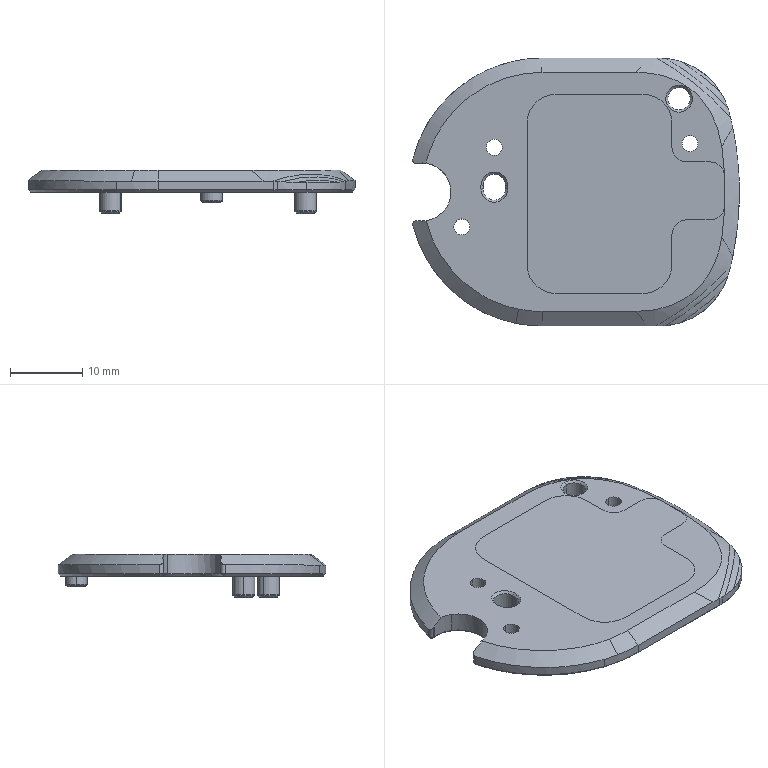NC program | NX | posted with a generic post | part box 45.101 x 36.973 x 6 mm
Lines 1 to 1808 of 5084, first 1683 of 1794 lines:
N10 G17 G21 G94 G90
(FLOOR_WALL_COPY_COPY , TOOL : D80)
N12 T19 M6
N14 G54
N16 G17 G0 G90 X-67.55 Y0. S6500 M3
N18 G43 Z30. H19
N20 Z6.
N22 G94 G1 Z3. F1500.
N24 X-62.55
N26 X62.55
N28 X67.55
N30 Z6.
N32 G0 Z30.
N34 X-67.55
N36 Z5.
N38 G1 Z2.
N40 X-62.55
N42 X62.55
N44 X67.55
N46 Z5.
N48 G0 Z30.
N50 X-67.55
N52 Z4.
N54 G1 Z1.
N56 X-62.55
N58 X62.55
N60 X67.55
N62 Z4.
N64 G0 Z30.
N66 X-67.55
N68 Z3.
N70 G1 Z0.
N72 X-62.55
N74 X62.55
N76 X67.55
N78 Z3.
N80 G0 Z30.
N82 M5
(CAVITY_MILL , TOOL : D6)
N84 T12 M6
N86 G54
N88 G17 G0 G90 X0.167 Y22.684 S9500 M3
N90 G43 Z30. H12
N92 Z0.65
N94 G94 G1 Z-0.35 F1000.
N96 Y18.831
N98 G3 X0.379 Y18.784 R0.5
N100 G1 X15.035 F3000.
N102 G2 X22.848 Y11.359 R21.5
N104 G1 Y1.003
N106 G2 X21.428 Y0.967 R3.5
N108 G3 X21.428 Y-1.001 R-1.
N110 G2 X22.848 Y-1.038 R3.5
N112 G1 Y-11.39
N114 G2 X15.091 Y-18.784 R21.5
N116 G1 X-19.432
N118 G2 X-22.848 Y-14.792 R13.
N120 G1 Y14.761
N122 G2 X-19.395 Y18.784 R13.
N124 G1 X0.379
N126 Y15.184
N128 X14.057
N130 G2 X19.248 Y10.277 R17.9
N132 G1 Y4.124
N134 G3 X19.248 Y-4.158 R4.6
N136 G1 Y-10.308
N138 G2 X14.107 Y-15.184 R17.9
N140 G1 X13.847
N142 G3 X8.65 Y-15.184 R-5.318
N144 G1 X9.002 Y-14.556
N146 G2 X7.237 Y-8.297 R4.598
N148 X9.002 Y-14.556 R-4.598
N150 G1 X8.65 Y-15.184
N152 X-18.086
N154 G2 X-19.248 Y-13.784 R9.4
N156 G1 Y-11.086
N158 G3 X-11.16 Y-9.945 R5.318
N160 X-10.588 Y-8.675 R5.318
N162 G1 X-10.437 Y-8.039
N164 G3 X-10.406 Y-7.825 R5.318
N166 G1 X-10.362 Y-7.253
N168 G3 X-19.248 Y-3.199 R5.318
N170 G1 X-18.765 Y-3.733
N172 G2 X-11.082 Y-7.238 R4.598
N174 G1 X-11.124 Y-7.769
N176 X-11.147 Y-7.917
N178 X-11.288 Y-8.507
N180 G2 X-18.765 Y-3.733 R-4.598
N182 G1 X-19.248 Y-3.199
N184 Y13.753
N186 G2 X-18.057 Y15.184 R9.4
N188 G1 X0.379
N190 Y11.584
N192 X12.966
N194 G2 X15.648 Y9.068 R14.3
N196 G1 Y5.97
N198 G3 X13.259 Y-1.855 R8.2
N200 X2.391 Y-11.584 R8.918
N202 G1 X-7.946
N204 G3 X-7.111 Y-9.612 R8.918
N206 G1 X-6.932 Y-8.867
N208 X-6.899 Y-8.704
N210 G3 X-6.837 Y-8.306 R8.918
N212 G1 X-6.821 Y-8.161
N214 X-6.771 Y-7.526
N216 X-6.764 Y-7.381
N218 G3 X-6.762 Y-7.013 R8.918
N220 X-15.648 Y1.776 R8.918
N222 G1 Y11.584
N224 X0.379
N226 Y7.984
N228 X11.709
N230 G2 X12.048 Y7.67 R10.7
N232 G1 Y7.368
N234 G3 X9.602 Y1.866 R11.8
N236 X-1.005 Y-7.984 R12.518
N238 G1 X-3.196
N240 X-3.178 Y-7.758
N242 X-3.166 Y-7.518
N244 G3 X-3.162 Y-6.959 R12.518
N246 X-12.048 Y4.838 R12.518
N248 G1 Y7.984
N250 X0.379
N252 Y4.384
N254 X5.17
N256 G3 X-1.126 Y-0.215 R16.118
N258 X-4.412 Y4.384 R16.118
N260 G1 X0.379
N262 G3 X1.145 Y4.741 R1.
N264 G1 Z0.65
N266 G0 Z30.
N268 X0.166 Y22.684
N270 Z0.3
N272 G1 Z-0.7 F1000.
N274 Y18.831
N276 G3 X0.378 Y18.784 R0.5
N278 G1 X15.035 F3000.
N280 G2 X22.848 Y11.359 R21.5
N282 G1 Y1.003
N284 G2 X21.428 Y0.967 R3.5
N286 G3 X21.428 Y-1.001 R-1.
N288 G2 X22.848 Y-1.038 R3.5
N290 G1 Y-11.39
N292 G2 X15.09 Y-18.784 R21.5
N294 G1 X-19.432
N296 G2 X-22.848 Y-14.792 R13.
N298 G1 Y14.761
N300 G2 X-19.395 Y18.784 R13.
N302 G1 X0.378
N304 Y15.184
N306 X14.057
N308 G2 X19.248 Y10.277 R17.9
N310 G1 Y4.124
N312 G3 X19.248 Y-4.158 R4.6
N314 G1 Y-10.308
N316 G2 X14.107 Y-15.184 R17.9
N318 G1 X13.85
N320 G3 X8.647 Y-15.184 R-5.32
N322 G1 X8.999 Y-14.556
N324 G2 X7.236 Y-8.294 R4.6
N326 X8.999 Y-14.556 R-4.6
N328 G1 X8.647 Y-15.184
N330 X-18.086
N332 G2 X-19.248 Y-13.783 R9.4
N334 G1 Y-11.088
N336 G3 X-19.248 Y-3.196 R-5.32
N338 G1 X-18.765 Y-3.73
N340 G2 X-12.268 Y-4.057 R4.6
N342 X-18.765 Y-3.73 R-4.6
N344 G1 X-19.248 Y-3.196
N346 Y13.753
N348 G2 X-18.056 Y15.184 R9.4
N350 G1 X0.378
N352 Y11.584
N354 X12.966
N356 G2 X15.648 Y9.068 R14.3
N358 G1 Y5.97
N360 G3 X13.259 Y-1.853 R8.2
N362 X2.389 Y-11.584 R8.92
N364 G1 X-7.944
N366 G3 X-15.648 Y1.778 R8.92
N368 G1 Y11.584
N370 X0.378
N372 Y7.984
N374 X11.709
N376 G2 X12.048 Y7.67 R10.7
N378 G1 Y7.369
N380 G3 X9.602 Y1.867 R11.8
N382 X-1.007 Y-7.984 R12.52
N384 G1 X-3.188
N386 G3 X-12.048 Y4.84 R12.52
N388 G1 Y7.984
N390 X0.378
N392 Y4.384
N394 X5.165
N396 G3 X-1.125 Y-0.212 R16.12
N398 X-4.41 Y4.384 R16.12
N400 G1 X0.378
N402 G3 X1.144 Y4.741 R1.
N404 G1 Z0.3
N406 G0 X0.166 Y22.684 Z-0.05
N408 G1 Z-1.05 F1000.
N410 Y18.831
N412 G3 X0.378 Y18.784 R0.5
N414 G1 X15.035 F3000.
N416 G2 X22.848 Y11.359 R21.5
N418 G1 Y1.003
N420 G2 X21.428 Y0.967 R3.5
N422 G3 X21.428 Y-1.001 R-1.
N424 G2 X22.848 Y-1.038 R3.5
N426 G1 Y-11.39
N428 G2 X15.09 Y-18.784 R21.5
N430 G1 X-19.432
N432 G2 X-22.848 Y-14.791 R13.
N434 G1 Y14.761
N436 G2 X-19.395 Y18.784 R13.
N438 G1 X0.378
N440 Y15.184
N442 X14.057
N444 G2 X19.248 Y10.277 R17.9
N446 G1 Y4.124
N448 G3 X19.248 Y-4.159 R4.6
N450 G1 Y-10.308
N452 G2 X14.106 Y-15.184 R17.9
N454 G1 X13.85
N456 G3 X8.647 Y-15.184 R-5.32
N458 G1 X8.999 Y-14.556
N460 G2 X7.236 Y-8.294 R4.6
N462 X8.999 Y-14.556 R-4.6
N464 G1 X8.647 Y-15.184
N466 X-18.086
N468 G2 X-19.248 Y-13.783 R9.4
N470 G1 Y-11.088
N472 G3 X-19.248 Y-3.197 R-5.32
N474 G1 X-18.765 Y-3.731
N476 G2 X-12.268 Y-4.057 R4.6
N478 X-18.765 Y-3.731 R-4.6
N480 G1 X-19.248 Y-3.197
N482 Y13.753
N484 G2 X-18.056 Y15.184 R9.4
N486 G1 X0.378
N488 Y11.584
N490 X12.966
N492 G2 X15.648 Y9.067 R14.3
N494 G1 Y5.97
N496 G3 X13.259 Y-1.853 R8.2
N498 X2.389 Y-11.584 R8.92
N500 G1 X-7.944
N502 G3 X-15.648 Y1.778 R8.92
N504 G1 Y11.584
N506 X0.378
N508 Y7.984
N510 X11.709
N512 G2 X12.048 Y7.67 R10.7
N514 G1 Y7.369
N516 G3 X9.602 Y1.867 R11.8
N518 X-1.007 Y-7.984 R12.52
N520 G1 X-3.188
N522 G3 X-12.048 Y4.84 R12.52
N524 G1 Y7.984
N526 X0.378
N528 Y4.384
N530 X5.165
N532 G3 X-1.125 Y-0.212 R16.12
N534 X-4.41 Y4.384 R16.12
N536 G1 X0.378
N538 G3 X1.144 Y4.742 R1.
N540 G1 Z-0.05
N542 G0 X0.166 Y22.684 Z-0.4
N544 G1 Z-1.4 F1000.
N546 Y18.831
N548 G3 X0.378 Y18.784 R0.5
N550 G1 X15.034 F3000.
N552 G2 X22.848 Y11.358 R21.5
N554 G1 Y1.003
N556 G2 X21.428 Y0.967 R3.5
N558 G3 X21.428 Y-1.001 R-1.
N560 G2 X22.848 Y-1.038 R3.5
N562 G1 Y-11.389
N564 G2 X15.09 Y-18.784 R21.5
N566 G1 X-19.432
N568 G2 X-22.848 Y-14.791 R13.
N570 G1 Y14.76
N572 G2 X-19.394 Y18.784 R13.
N574 G1 X0.378
N576 Y15.184
N578 X14.057
N580 G2 X19.248 Y10.277 R17.9
N582 G1 Y4.124
N584 G3 X19.248 Y-4.159 R4.6
N586 G1 Y-10.308
N588 G2 X14.106 Y-15.184 R17.9
N590 G1 X13.85
N592 G3 X8.647 Y-15.184 R-5.32
N594 G1 X8.999 Y-14.556
N596 G2 X7.236 Y-8.295 R4.6
N598 X8.999 Y-14.556 R-4.6
N600 G1 X8.647 Y-15.184
N602 X-18.086
N604 G2 X-19.248 Y-13.783 R9.4
N606 G1 Y-11.088
N608 G3 X-19.248 Y-3.197 R-5.32
N610 G1 X-18.765 Y-3.731
N612 G2 X-12.268 Y-4.056 R4.6
N614 X-18.765 Y-3.731 R-4.6
N616 G1 X-19.248 Y-3.197
N618 Y13.753
N620 G2 X-18.056 Y15.184 R9.4
N622 G1 X0.378
N624 Y11.584
N626 X12.966
N628 G2 X15.648 Y9.067 R14.3
N630 G1 Y5.97
N632 G3 X13.259 Y-1.853 R8.2
N634 X2.389 Y-11.584 R8.92
N636 G1 X-7.944
N638 G3 X-15.648 Y1.778 R8.92
N640 G1 Y11.584
N642 X0.378
N644 Y7.984
N646 X11.709
N648 G2 X12.048 Y7.67 R10.7
N650 G1 Y7.369
N652 G3 X9.602 Y1.867 R11.8
N654 X-1.007 Y-7.984 R12.52
N656 G1 X-3.188
N658 G3 X-12.048 Y4.84 R12.52
N660 G1 Y7.984
N662 X0.378
N664 Y4.384
N666 X5.166
N668 G3 X-1.125 Y-0.212 R16.12
N670 X-4.41 Y4.384 R16.12
N672 G1 X0.378
N674 G3 X1.144 Y4.742 R1.
N676 G1 Z-0.4
N678 G0 X-1.96 Y-22.685 Z-0.775
N680 G1 Z-1.775 F1000.
N682 Y-18.831
N684 G3 X-2.171 Y-18.785 R0.5
N686 G1 X-19.431 F3000.
N688 G2 X-22.848 Y-14.791 R13.
N690 G1 Y14.76
N692 G2 X-19.394 Y18.785 R13.
N694 G1 X-7.207
N696 G2 X1.794 Y18.785 R5.3
N698 G1 X15.034
N700 G2 X22.848 Y11.358 R21.5
N702 G1 Y1.003
N704 G2 X21.428 Y0.967 R3.5
N706 G3 X21.428 Y-1.001 R-1.
N708 G2 X22.848 Y-1.038 R3.5
N710 G1 Y-11.389
N712 G2 X15.09 Y-18.785 R21.5
N714 G1 X-2.171
N716 Y-15.185
N718 X-18.086
N720 G2 X-19.248 Y-13.783 R9.4
N722 G1 Y-11.088
N724 G3 X-19.248 Y-3.197 R-5.32
N726 G1 X-18.765 Y-3.731
N728 G2 X-12.268 Y-4.056 R4.6
N730 X-18.765 Y-3.731 R-4.6
N732 G1 X-19.248 Y-3.197
N734 Y13.753
N736 G2 X-18.056 Y15.185 R9.4
N738 G1 X-7.946
N740 G3 X2.533 Y15.185 R5.3
N742 G1 X1.821 Y15.293
N744 G2 X-3.398 Y11.458 R4.58
N746 X1.821 Y15.293 R-4.58
N748 G1 X2.533 Y15.185
N750 X14.056
N752 G2 X19.248 Y10.276 R17.9
N754 G1 Y4.124
N756 G3 X19.248 Y-4.159 R4.6
N758 G1 Y-10.307
N760 G2 X14.106 Y-15.185 R17.9
N762 G1 X13.85
N764 G3 X8.647 Y-15.185 R-5.32
N766 G1 X8.999 Y-14.557
N768 G2 X7.236 Y-8.295 R4.6
N770 X8.999 Y-14.557 R-4.6
N772 G1 X8.647 Y-15.185
N774 X-2.171
N776 Y-11.585
N778 X-7.944
N780 G3 X-15.648 Y1.778 R8.92
N782 G1 Y11.585
N784 X-10.443
N786 G3 X5.029 Y11.585 R8.9
N788 G1 X12.965
N790 G2 X15.648 Y9.067 R14.3
N792 G1 Y5.971
N794 G3 X13.259 Y-1.853 R8.2
N796 X2.389 Y-11.585 R8.92
N798 G1 X-2.171
N800 Y-7.985
N802 X-3.188
N804 G3 X-12.048 Y4.84 R12.52
N806 G1 Y7.68
N808 G3 X6.898 Y7.985 R12.5
N810 G1 X11.709
N812 G2 X12.048 Y7.669 R10.7
N814 G1 Y7.369
N816 G3 X9.602 Y1.867 R11.8
N818 X-1.007 Y-7.985 R12.52
N820 G1 X-2.171
N822 X-1.125 Y-0.212
N824 X-1.206 Y-0.045
N826 G3 X-0.962 Y-0.02 R16.1
N828 X-1.125 Y-0.212 R16.12
N830 X-1.342 Y-1.029 R1.
N832 G1 Z-0.775
N834 G0 X-1.96 Y-22.685 Z-1.15
N836 G1 Z-2.15 F1000.
N838 Y-18.832
N840 G3 X-2.171 Y-18.785 R0.5
N842 G1 X-19.431 F3000.
N844 G2 X-22.849 Y-14.79 R13.
N846 G1 Y14.76
N848 G2 X-19.394 Y18.785 R13.
N850 G1 X-7.23
N852 G2 X1.817 Y18.785 R5.32
N854 G1 X15.034
N856 G2 X22.849 Y11.358 R21.5
N858 G1 Y1.003
N860 G2 X21.428 Y0.967 R3.5
N862 G3 X21.428 Y-1.001 R-1.
N864 G2 X22.849 Y-1.038 R3.5
N866 G1 Y-11.389
N868 G2 X15.089 Y-18.785 R21.5
N870 G1 X-2.171
N872 Y-15.185
N874 X-18.085
N876 G2 X-19.249 Y-13.782 R9.4
N878 G1 Y-11.088
N880 G3 X-19.249 Y-3.197 R-5.32
N882 G1 X-18.766 Y-3.731
N884 G2 X-12.268 Y-4.056 R4.6
N886 X-18.766 Y-3.731 R-4.6
N888 G1 X-19.249 Y-3.197
N890 Y13.752
N892 G2 X-18.056 Y15.185 R9.4
N894 G1 X-7.966
N896 G3 X2.553 Y15.185 R5.32
N898 G1 X1.841 Y15.293
N900 G2 X-3.399 Y11.437 R4.6
N902 X1.841 Y15.293 R-4.6
N904 G1 X2.553 Y15.185
N906 X14.056
N908 G2 X19.249 Y10.276 R17.9
N910 G1 Y4.124
N912 G3 X19.249 Y-4.159 R4.6
N914 G1 Y-10.307
N916 G2 X14.106 Y-15.185 R17.9
N918 G1 X13.849
N920 G3 X8.648 Y-15.185 R-5.32
N922 G1 X9. Y-14.557
N924 G2 X7.236 Y-8.295 R4.6
N926 X9. Y-14.557 R-4.6
N928 G1 X8.648 Y-15.185
N930 X-2.171
N932 Y-11.585
N934 X-7.944
N936 G3 X-15.649 Y1.778 R8.92
N938 G1 Y11.585
N940 X-10.466
N942 G3 X5.053 Y11.585 R8.92
N944 G1 X12.965
N946 G2 X15.649 Y9.067 R14.3
N948 G1 Y5.971
N950 G3 X13.259 Y-1.853 R8.2
N952 X2.389 Y-11.585 R8.92
N954 G1 X-2.171
N956 Y-7.985
N958 X-3.188
N960 G3 X-12.049 Y4.84 R12.52
N962 G1 Y7.65
N964 G3 X6.924 Y7.985 R12.52
N966 G1 X11.708
N968 G2 X12.049 Y7.669 R10.7
N970 G1 Y7.369
N972 G3 X9.602 Y1.867 R11.8
N974 X-1.007 Y-7.985 R12.52
N976 G1 X-2.171
N978 X-1.125 Y-0.212
N980 X-1.196 Y-0.064
N982 G3 X-0.982 Y-0.042 R16.12
N984 X-1.125 Y-0.212 R16.12
N986 X-1.342 Y-1.029 R1.
N988 G1 Z-1.15
N990 G0 X-1.96 Y-22.685 Z-1.525
N992 G1 Z-2.525 F1000.
N994 Y-18.832
N996 G3 X-2.171 Y-18.785 R0.5
N998 G1 X-19.431 F3000.
N1000 G2 X-22.849 Y-14.79 R13.
N1002 G1 Y14.759
N1004 G2 X-19.394 Y18.785 R13.
N1006 G1 X-7.23
N1008 G2 X1.817 Y18.785 R5.32
N1010 G1 X15.034
N1012 G2 X22.849 Y11.358 R21.5
N1014 G1 Y1.003
N1016 G2 X21.428 Y0.967 R3.5
N1018 G3 X21.428 Y-1.001 R-1.
N1020 G2 X22.849 Y-1.038 R3.5
N1022 G1 Y-11.388
N1024 G2 X15.089 Y-18.785 R21.5
N1026 G1 X-2.171
N1028 Y-15.185
N1030 X-18.085
N1032 G2 X-19.249 Y-13.782 R9.4
N1034 G1 Y-11.087
N1036 G3 X-19.249 Y-3.197 R-5.32
N1038 G1 X-18.766 Y-3.731
N1040 G2 X-12.268 Y-4.056 R4.6
N1042 X-18.766 Y-3.731 R-4.6
N1044 G1 X-19.249 Y-3.197
N1046 Y13.752
N1048 G2 X-18.056 Y15.185 R9.4
N1050 G1 X-7.966
N1052 G3 X2.553 Y15.185 R5.32
N1054 G1 X1.841 Y15.293
N1056 G2 X-3.398 Y11.437 R4.6
N1058 X1.841 Y15.293 R-4.6
N1060 G1 X2.553 Y15.185
N1062 X14.056
N1064 G2 X19.249 Y10.276 R17.9
N1066 G1 Y4.124
N1068 G3 X19.249 Y-4.159 R4.6
N1070 G1 Y-10.307
N1072 G2 X14.106 Y-15.185 R17.9
N1074 G1 X13.849
N1076 G3 X8.648 Y-15.185 R-5.32
N1078 G1 X9. Y-14.557
N1080 G2 X7.236 Y-8.295 R4.6
N1082 X9. Y-14.557 R-4.6
N1084 G1 X8.648 Y-15.185
N1086 X-2.171
N1088 Y-11.585
N1090 X-7.944
N1092 G3 X-15.649 Y1.778 R8.92
N1094 G1 Y11.585
N1096 X-10.466
N1098 G3 X5.053 Y11.585 R8.92
N1100 G1 X12.965
N1102 G2 X15.649 Y9.067 R14.3
N1104 G1 Y5.971
N1106 G3 X13.259 Y-1.853 R8.2
N1108 X2.389 Y-11.585 R8.92
N1110 G1 X-2.171
N1112 Y-7.985
N1114 X-3.188
N1116 G3 X-12.049 Y4.84 R12.52
N1118 G1 Y7.65
N1120 G3 X6.924 Y7.985 R12.52
N1122 G1 X11.708
N1124 G2 X12.049 Y7.669 R10.7
N1126 G1 Y7.37
N1128 G3 X9.602 Y1.867 R11.8
N1130 X-1.007 Y-7.985 R12.52
N1132 G1 X-2.171
N1134 X-1.125 Y-0.212
N1136 X-1.196 Y-0.064
N1138 G3 X-0.982 Y-0.042 R16.12
N1140 X-1.125 Y-0.212 R16.12
N1142 X-1.342 Y-1.029 R1.
N1144 G1 Z-1.525
N1146 G0 X-1.96 Y-22.685 Z-1.9
N1148 G1 Z-2.9 F1000.
N1150 Y-18.832
N1152 G3 X-2.171 Y-18.785 R0.5
N1154 G1 X-19.431 F3000.
N1156 G2 X-22.849 Y-14.79 R13.
N1158 G1 Y14.759
N1160 G2 X-19.394 Y18.785 R13.
N1162 G1 X-7.23
N1164 G2 X1.817 Y18.785 R5.32
N1166 G1 X15.033
N1168 G2 X22.849 Y11.357 R21.5
N1170 G1 Y1.003
N1172 G2 X21.428 Y0.967 R3.5
N1174 G3 X21.428 Y-1.001 R-1.
N1176 G2 X22.849 Y-1.038 R3.5
N1178 G1 Y-11.388
N1180 G2 X15.089 Y-18.785 R21.5
N1182 G1 X-2.171
N1184 Y-15.185
N1186 X-18.085
N1188 G2 X-19.249 Y-13.782 R9.4
N1190 G1 Y-11.087
N1192 G3 X-19.249 Y-3.197 R-5.32
N1194 G1 X-18.766 Y-3.731
N1196 G2 X-12.268 Y-4.056 R4.6
N1198 X-18.766 Y-3.731 R-4.6
N1200 G1 X-19.249 Y-3.197
N1202 Y13.752
N1204 G2 X-18.056 Y15.185 R9.4
N1206 G1 X-7.966
N1208 G3 X2.553 Y15.185 R5.32
N1210 G1 X1.841 Y15.293
N1212 G2 X-3.398 Y11.437 R4.6
N1214 X1.841 Y15.293 R-4.6
N1216 G1 X2.553 Y15.185
N1218 X14.056
N1220 G2 X19.249 Y10.276 R17.9
N1222 G1 Y4.124
N1224 G3 X19.249 Y-4.159 R4.6
N1226 G1 Y-10.307
N1228 G2 X14.105 Y-15.185 R17.9
N1230 G1 X13.849
N1232 G3 X8.648 Y-15.185 R-5.32
N1234 G1 X9. Y-14.557
N1236 G2 X7.235 Y-8.295 R4.6
N1238 X9. Y-14.557 R-4.6
N1240 G1 X8.648 Y-15.185
N1242 X-2.171
N1244 Y-11.585
N1246 X-7.944
N1248 G3 X-15.649 Y1.778 R8.92
N1250 G1 Y11.585
N1252 X-10.466
N1254 G3 X5.053 Y11.585 R8.92
N1256 G1 X12.965
N1258 G2 X15.649 Y9.066 R14.3
N1260 G1 Y5.971
N1262 G3 X13.259 Y-1.853 R8.2
N1264 X2.389 Y-11.585 R8.92
N1266 G1 X-2.171
N1268 Y-7.985
N1270 X-3.188
N1272 G3 X-12.049 Y4.84 R12.52
N1274 G1 Y7.65
N1276 G3 X6.924 Y7.985 R12.52
N1278 G1 X11.708
N1280 G2 X12.049 Y7.669 R10.7
N1282 G1 Y7.37
N1284 G3 X9.602 Y1.867 R11.8
N1286 X-1.007 Y-7.985 R12.52
N1288 G1 X-2.171
N1290 X-1.125 Y-0.212
N1292 X-1.196 Y-0.064
N1294 G3 X-0.982 Y-0.042 R16.12
N1296 X-1.125 Y-0.212 R16.12
N1298 X-1.342 Y-1.029 R1.
N1300 G1 Z-1.9
N1302 G0 X-3.718 Y-2.069 Z-1.4
N1304 G1 X-3.562 Y-2.478 Z-1.423 F1000.
N1306 X-3.384 Y-3.313 Z-1.468
N1308 Y3.351 Z-1.817
N1310 X-3.443 Z-1.82
N1312 X-3.641 Y2.52 Z-1.865
N1314 X-4.281 Y0.893 Z-1.956
N1316 X-4.703 Y0.151 Z-2.001
N1318 X-4.281 Y-0.591 Z-2.046
N1320 X-3.562 Y-2.478 Z-2.152
N1322 X-3.384 Y-3.313 Z-2.197
N1324 Y3.351 Z-2.546
N1326 X-3.443 Z-2.549
N1328 X-3.641 Y2.52 Z-2.594
N1330 X-4.281 Y0.893 Z-2.685
N1332 X-4.703 Y0.151 Z-2.73
N1334 X-4.281 Y-0.591 Z-2.775
N1336 X-3.562 Y-2.478 Z-2.881
N1338 X-3.384 Y-3.313 Z-2.925
N1340 Y0.019 Z-3.1
N1342 Y3.351 F3000.
N1344 X-3.443
N1346 G2 X-4.703 Y0.151 R12.134
N1348 X-3.384 Y-3.313 R12.134
N1350 G1 Y0.019
N1352 X0.216
N1354 Y6.951
N1356 X-6.716
N1358 Y6.151
N1360 G2 X-9.181 Y0.151 R8.534
N1362 X-6.716 Y-5.849 R8.534
N1364 G1 Y-7.937
N1366 G2 X-4.182 Y-7.481 R7.006
N1368 G1 X0.216
N1370 Y0.019
N1372 X3.816
N1374 Y9.475
N1376 G3 X2.733 Y10.551 R1.066
N1378 G1 X-9.24
N1380 G3 X-10.316 Y9.485 R1.066
N1382 G1 Y6.151
N1384 G2 X-15.25 Y1.217 R4.934
N1386 G1 X-17.58 Y1.218
N1388 Y-0.914
N1390 X-15.249 Y-0.915
N1392 G2 X-10.316 Y-5.849 R4.934
N1394 G1 Y-10.015
N1396 X-10.277 Y-10.483
N1398 G2 X-12.204 Y-13.802 R3.352
N1400 G1 X-7.551 Y-13.731
N1402 G2 X-4.196 Y-11.081 R3.406
N1404 G1 X2.75
N1406 G3 X3.816 Y-10.034 R1.066
N1408 G1 Y0.019
N1410 G3 X3.459 Y0.785 R1.
N1412 G1 Z-2.1
N1414 G0 X-3.55 Y1.045 Z-1.6
N1416 G1 Y2.357 Z-1.669 F1000.
N1418 X-3.815 Y1.539 Z-1.714
N1420 X-4.093 Y0.902 Z-1.75
N1422 X-4.512 Y0.151 Z-1.795
N1424 X-4.093 Y-0.599 Z-1.84
N1426 X-3.815 Y-1.236 Z-1.877
N1428 X-3.55 Y-2.054 Z-1.922
N1430 Y2.357 Z-2.153
N1432 X-3.815 Y1.539 Z-2.198
N1434 X-4.093 Y0.902 Z-2.234
N1436 X-4.512 Y0.151 Z-2.279
N1438 X-4.093 Y-0.599 Z-2.325
N1440 X-3.815 Y-1.236 Z-2.361
N1442 X-3.55 Y-2.054 Z-2.406
N1444 Y2.357 Z-2.637
N1446 X-3.815 Y1.539 Z-2.682
N1448 X-4.093 Y0.902 Z-2.719
N1450 X-4.512 Y0.151 Z-2.764
N1452 X-4.093 Y-0.599 Z-2.809
N1454 X-3.815 Y-1.236 Z-2.845
N1456 X-3.55 Y-2.054 Z-2.89
N1458 Y2.357 Z-3.121
N1460 X-3.815 Y1.539 Z-3.166
N1462 X-4.093 Y0.902 Z-3.203
N1464 X-4.512 Y0.151 Z-3.248
N1466 X-4.093 Y-0.599 Z-3.293
N1468 X-3.815 Y-1.236 Z-3.329
N1470 X-3.55 Y-2.054 Z-3.374
N1472 Y0.151 Z-3.49
N1474 Y2.357 F3000.
N1476 G2 X-4.512 Y0.151 R12.3
N1478 X-3.55 Y-2.054 R12.3
N1480 G1 Y0.151
N1482 X0.05
N1484 Y6.785
N1486 X-6.55
N1488 Y6.141
N1490 G2 X-8.95 Y0.151 R8.7
N1492 X-6.55 Y-5.836 R8.7
N1494 G1 Y-7.684
N1496 G2 X-4.443 Y-7.316 R6.995
N1498 G1 X0.05 Y-7.315
N1500 Y0.151
N1502 X3.65
N1504 Y9.485
N1506 G3 X2.75 Y10.385 R0.9
N1508 G1 X-9.25
N1510 G3 X-10.15 Y9.485 R0.9
N1512 G1 Y6.143
N1514 G2 X-15.25 Y1.051 R5.1
N1516 G1 X-17.414 Y1.052
N1518 Y-0.748
N1520 X-15.233 Y-0.749
N1522 G2 X-10.15 Y-5.84 R5.1
N1524 G1 Y-10.015
N1526 X-10.134 Y-10.184
N1528 G2 X-11.381 Y-13.565 R3.587
N1530 G1 X-7.742 Y-13.509
N1532 G2 X-6.644 Y-11.847 R3.168
N1534 X-4.373 Y-10.915 R3.395
N1536 G1 X2.75
N1538 G3 X3.65 Y-10.015 R0.9
N1540 G1 Y0.151
N1542 G3 X3.293 Y0.917 R1.
N1544 G1 Z-2.49
N1546 G0 X-3.55 Y1.045 Z-1.99
N1548 G1 Y2.357 Z-2.059 F1000.
N1550 X-3.815 Y1.539 Z-2.104
N1552 X-4.093 Y0.902 Z-2.14
N1554 X-4.512 Y0.151 Z-2.185
N1556 X-4.093 Y-0.599 Z-2.23
N1558 X-3.815 Y-1.236 Z-2.267
N1560 X-3.55 Y-2.054 Z-2.312
N1562 Y2.357 Z-2.543
N1564 X-3.815 Y1.539 Z-2.588
N1566 X-4.093 Y0.902 Z-2.624
N1568 X-4.512 Y0.151 Z-2.669
N1570 X-4.093 Y-0.599 Z-2.715
N1572 X-3.815 Y-1.236 Z-2.751
N1574 X-3.55 Y-2.054 Z-2.796
N1576 Y2.357 Z-3.027
N1578 X-3.815 Y1.539 Z-3.072
N1580 X-4.093 Y0.902 Z-3.109
N1582 X-4.512 Y0.151 Z-3.154
N1584 X-4.093 Y-0.599 Z-3.199
N1586 X-3.815 Y-1.236 Z-3.235
N1588 X-3.55 Y-2.054 Z-3.28
N1590 Y2.357 Z-3.511
N1592 X-3.815 Y1.539 Z-3.556
N1594 X-4.093 Y0.902 Z-3.593
N1596 X-4.512 Y0.151 Z-3.638
N1598 X-4.093 Y-0.599 Z-3.683
N1600 X-3.815 Y-1.236 Z-3.719
N1602 X-3.55 Y-2.054 Z-3.764
N1604 Y0.151 Z-3.88
N1606 Y2.357 F3000.
N1608 G2 X-4.512 Y0.151 R12.3
N1610 X-3.55 Y-2.054 R12.3
N1612 G1 Y0.151
N1614 X0.05
N1616 Y6.785
N1618 X-6.55
N1620 Y6.141
N1622 G2 X-8.95 Y0.151 R8.7
N1624 X-6.55 Y-5.836 R8.7
N1626 G1 Y-7.611
N1628 G2 X-5.145 Y-7.339 R8.161
N1630 G1 X0.05 Y-7.315
N1632 Y0.151
N1634 X3.65
N1636 Y9.485
N1638 G3 X2.75 Y10.385 R0.9
N1640 G1 X-9.25
N1642 G3 X-10.15 Y9.485 R0.9
N1644 G1 Y6.143
N1646 G2 X-15.25 Y1.051 R5.1
N1648 G1 X-17.414 Y1.052
N1650 Y-0.748
N1652 X-15.233 Y-0.749
N1654 G2 X-10.15 Y-5.84 R5.1
N1656 G1 Y-10.015
N1658 G3 X-10.122 Y-10.236 R0.9
N1660 G2 X-10.112 Y-11.963 R3.522
N1662 G1 X-10.333 Y-12.923
N1664 X-8.076 Y-12.888
N1666 G2 X-4.847 Y-10.929 R4.561
N1668 G1 X-4.548 Y-10.915
N1670 X2.75
N1672 G3 X3.65 Y-10.015 R0.9
N1674 G1 Y0.151
N1676 G3 X3.293 Y0.917 R1.
N1678 G1 Z-2.88
N1680 G0 X-3.939 Y1.255 Z-2.38
N1682 G1 X-4.093 Y0.902 Z-2.4 F1000.
N1684 X-4.512 Y0.151 Z-2.445
N1686 X-4.093 Y-0.599 Z-2.49
N1688 X-3.815 Y-1.236 Z-2.527
N1690 X-3.55 Y-2.054 Z-2.572
N1692 Y2.357 Z-2.803
N1694 X-3.815 Y1.539 Z-2.848
N1696 X-4.093 Y0.902 Z-2.884
N1698 X-4.512 Y0.151 Z-2.929
N1700 X-4.093 Y-0.599 Z-2.975
N1702 X-3.815 Y-1.236 Z-3.011
N1704 X-3.55 Y-2.054 Z-3.056
N1706 Y2.357 Z-3.287
N1708 X-3.815 Y1.539 Z-3.332
N1710 X-4.093 Y0.902 Z-3.369
N1712 X-4.512 Y0.151 Z-3.414
N1714 X-4.093 Y-0.599 Z-3.459
N1716 X-3.815 Y-1.236 Z-3.495
N1718 X-3.55 Y-2.054 Z-3.54
N1720 Y2.357 Z-3.771
N1722 X-3.815 Y1.539 Z-3.816
N1724 X-4.093 Y0.902 Z-3.853
N1726 X-4.512 Y0.151 Z-3.898
N1728 X-4.093 Y-0.599 Z-3.943
N1730 X-3.815 Y-1.236 Z-3.979
N1732 X-3.55 Y-2.054 Z-4.024
N1734 Y0.151 Z-4.14
N1736 Y2.357 F3000.
N1738 G2 X-4.512 Y0.151 R12.3
N1740 X-3.55 Y-2.054 R12.3
N1742 G1 Y0.151
N1744 X0.05
N1746 Y6.785
N1748 X-6.55
N1750 Y6.141
N1752 G2 X-8.95 Y0.151 R8.7
N1754 X-6.55 Y-5.836 R8.7
N1756 G1 Y-7.414
N1758 X-6.138
N1760 X-5.009 Y-7.315
N1762 X0.05
N1764 Y0.151
N1766 X3.65
N1768 Y9.485
N1770 G3 X2.75 Y10.385 R0.9
N1772 G1 X-9.25
N1774 G3 X-10.15 Y9.485 R0.9
N1776 G1 Y6.143
N1778 G2 X-15.25 Y1.051 R5.1
N1780 G1 X-17.414 Y1.052
N1782 Y-0.748
N1784 X-15.233 Y-0.749
N1786 G2 X-10.15 Y-5.84 R5.1
N1788 G1 Y-10.015
N1790 G3 X-10.106 Y-10.301 R0.903
N1792 G1 X-9.993 Y-10.682
N1794 G3 X-9.25 Y-11.014 R1.012
N1796 G1 X-5.981
N1798 X-4.852 Y-10.915
N1800 X2.75
N1802 G3 X3.65 Y-10.015 R0.9
N1804 G1 Y0.151
N1806 G3 X3.293 Y0.917 R1.
N1808 G1 Z-3.14
N1810 G0 X-3.939 Y1.255 Z-2.64
N1812 G1 X-4.093 Y0.902 Z-2.66 F1000.
N1814 X-4.512 Y0.151 Z-2.705
N1816 X-4.093 Y-0.599 Z-2.75
N1818 X-3.815 Y-1.236 Z-2.787
N1820 X-3.55 Y-2.054 Z-2.832
N1822 Y2.357 Z-3.063
N1824 X-3.815 Y1.539 Z-3.108
N1826 X-4.093 Y0.902 Z-3.144
N1828 X-4.512 Y0.151 Z-3.189
N1830 X-4.093 Y-0.599 Z-3.235
N1832 X-3.815 Y-1.236 Z-3.271
N1834 X-3.55 Y-2.054 Z-3.316
N1836 Y2.357 Z-3.547
N1838 X-3.815 Y1.539 Z-3.592
N1840 X-4.093 Y0.902 Z-3.629
N1842 X-4.512 Y0.151 Z-3.674
N1844 X-4.093 Y-0.599 Z-3.719
N1846 X-3.815 Y-1.236 Z-3.755
N1848 X-3.55 Y-2.054 Z-3.8
N1850 Y2.357 Z-4.031
N1852 X-3.815 Y1.539 Z-4.076
N1854 X-4.093 Y0.902 Z-4.113
N1856 X-4.512 Y0.151 Z-4.158
N1858 X-4.093 Y-0.599 Z-4.203
N1860 X-3.815 Y-1.236 Z-4.239
N1862 X-3.55 Y-2.054 Z-4.284
N1864 Y0.151 Z-4.4
N1866 Y2.357 F3000.
N1868 G2 X-4.512 Y0.151 R12.3
N1870 X-3.55 Y-2.054 R12.3
N1872 G1 Y0.151
N1874 X0.05
N1876 Y6.785
N1878 X-6.55
N1880 Y6.141
N1882 G2 X-8.95 Y0.151 R8.7
N1884 X-6.55 Y-5.836 R8.7
N1886 G1 Y-7.315
N1888 X0.05
N1890 Y0.151
N1892 X3.65
N1894 Y9.485
N1896 G3 X2.75 Y10.385 R0.9
N1898 G1 X-9.25
N1900 G3 X-10.15 Y9.485 R0.9
N1902 G1 Y6.143
N1904 G2 X-15.25 Y1.051 R5.1
N1906 G1 X-17.414 Y1.052
N1908 Y-0.748
N1910 X-15.233 Y-0.749
N1912 G2 X-10.15 Y-5.84 R5.1
N1914 G1 Y-10.015
N1916 G3 X-9.25 Y-10.915 R0.9
N1918 G1 X2.75
N1920 G3 X3.65 Y-10.015 R0.9
N1922 G1 Y0.151
N1924 G3 X3.293 Y0.917 R1.
N1926 G1 Z-3.4
N1928 G0 X-3.55 Y0.855 Z-2.9
N1930 G1 Y2.357 Z-2.979 F1000.
N1932 X-3.815 Y1.539 Z-3.024
N1934 X-4.093 Y0.902 Z-3.06
N1936 X-4.512 Y0.151 Z-3.105
N1938 X-4.093 Y-0.599 Z-3.15
N1940 X-3.815 Y-1.236 Z-3.187
N1942 X-3.55 Y-2.054 Z-3.232
N1944 Y2.357 Z-3.463
N1946 X-3.815 Y1.539 Z-3.508
N1948 X-4.093 Y0.902 Z-3.544
N1950 X-4.512 Y0.151 Z-3.589
N1952 X-4.093 Y-0.599 Z-3.635
N1954 X-3.815 Y-1.236 Z-3.671
N1956 X-3.55 Y-2.054 Z-3.716
N1958 Y2.357 Z-3.947
N1960 X-3.815 Y1.539 Z-3.992
N1962 X-4.093 Y0.902 Z-4.029
N1964 X-4.512 Y0.151 Z-4.074
N1966 X-4.093 Y-0.599 Z-4.119
N1968 X-3.815 Y-1.236 Z-4.155
N1970 X-3.55 Y-2.054 Z-4.2
N1972 Y2.357 Z-4.431
N1974 X-3.815 Y1.539 Z-4.476
N1976 X-4.093 Y0.902 Z-4.513
N1978 X-4.512 Y0.151 Z-4.558
N1980 X-4.093 Y-0.599 Z-4.603
N1982 X-3.815 Y-1.236 Z-4.639
N1984 X-3.55 Y-2.054 Z-4.684
N1986 Y0.151 Z-4.8
N1988 Y2.357 F3000.
N1990 G2 X-4.512 Y0.151 R12.3
N1992 X-3.55 Y-2.054 R12.3
N1994 G1 Y0.151
N1996 X0.05
N1998 Y6.785
N2000 X-6.55
N2002 Y6.141
N2004 G2 X-8.95 Y0.151 R8.7
N2006 X-6.55 Y-5.836 R8.7
N2008 G1 Y-7.315
N2010 X0.05
N2012 Y0.151
N2014 X3.65
N2016 Y9.485
N2018 G3 X2.75 Y10.385 R0.9
N2020 G1 X-9.25
N2022 G3 X-10.15 Y9.485 R0.9
N2024 G1 Y6.143
N2026 G2 X-15.25 Y1.051 R5.1
N2028 G1 X-17.414 Y1.052
N2030 Y-0.748
N2032 X-15.233 Y-0.749
N2034 G2 X-10.15 Y-5.84 R5.1
N2036 G1 Y-10.015
N2038 G3 X-9.25 Y-10.915 R0.9
N2040 G1 X2.75
N2042 G3 X3.65 Y-10.015 R0.9
N2044 G1 Y0.151
N2046 G3 X3.293 Y0.917 R1.
N2048 G1 Z-3.8
N2050 G0 X-3.55 Y0.855 Z-3.3
N2052 G1 Y2.357 Z-3.379 F1000.
N2054 X-3.815 Y1.539 Z-3.424
N2056 X-4.093 Y0.902 Z-3.46
N2058 X-4.512 Y0.151 Z-3.505
N2060 X-4.093 Y-0.599 Z-3.55
N2062 X-3.815 Y-1.236 Z-3.587
N2064 X-3.55 Y-2.054 Z-3.632
N2066 Y2.357 Z-3.863
N2068 X-3.815 Y1.539 Z-3.908
N2070 X-4.093 Y0.902 Z-3.944
N2072 X-4.512 Y0.151 Z-3.989
N2074 X-4.093 Y-0.599 Z-4.035
N2076 X-3.815 Y-1.236 Z-4.071
N2078 X-3.55 Y-2.054 Z-4.116
N2080 Y2.357 Z-4.347
N2082 X-3.815 Y1.539 Z-4.392
N2084 X-4.093 Y0.902 Z-4.429
N2086 X-4.512 Y0.151 Z-4.474
N2088 X-4.093 Y-0.599 Z-4.519
N2090 X-3.815 Y-1.236 Z-4.555
N2092 X-3.55 Y-2.054 Z-4.6
N2094 Y2.357 Z-4.831
N2096 X-3.815 Y1.539 Z-4.876
N2098 X-4.093 Y0.902 Z-4.913
N2100 X-4.512 Y0.151 Z-4.958
N2102 X-4.093 Y-0.599 Z-5.003
N2104 X-3.815 Y-1.236 Z-5.039
N2106 X-3.55 Y-2.054 Z-5.084
N2108 Y0.151 Z-5.2
N2110 Y2.357 F3000.
N2112 G2 X-4.512 Y0.151 R12.3
N2114 X-3.55 Y-2.054 R12.3
N2116 G1 Y0.151
N2118 X0.05
N2120 Y6.785
N2122 X-6.55
N2124 Y6.141
N2126 G2 X-8.95 Y0.151 R8.7
N2128 X-6.55 Y-5.836 R8.7
N2130 G1 Y-7.315
N2132 X0.05
N2134 Y0.151
N2136 X3.65
N2138 Y9.485
N2140 G3 X2.75 Y10.385 R0.9
N2142 G1 X-9.25
N2144 G3 X-10.15 Y9.485 R0.9
N2146 G1 Y6.143
N2148 G2 X-15.25 Y1.051 R5.1
N2150 G1 X-17.414 Y1.052
N2152 Y-0.748
N2154 X-15.233 Y-0.749
N2156 G2 X-10.15 Y-5.84 R5.1
N2158 G1 Y-10.015
N2160 G3 X-9.25 Y-10.915 R0.9
N2162 G1 X2.75
N2164 G3 X3.65 Y-10.015 R0.9
N2166 G1 Y0.151
N2168 G3 X3.293 Y0.917 R1.
N2170 G1 Z-4.2
N2172 G0 X-3.55 Y0.855 Z-3.7
N2174 G1 Y2.357 Z-3.779 F1000.
N2176 X-3.815 Y1.539 Z-3.824
N2178 X-4.093 Y0.902 Z-3.86
N2180 X-4.512 Y0.151 Z-3.905
N2182 X-4.093 Y-0.599 Z-3.95
N2184 X-3.815 Y-1.236 Z-3.987
N2186 X-3.55 Y-2.054 Z-4.032
N2188 Y2.357 Z-4.263
N2190 X-3.815 Y1.539 Z-4.308
N2192 X-4.093 Y0.902 Z-4.344
N2194 X-4.512 Y0.151 Z-4.389
N2196 X-4.093 Y-0.599 Z-4.435
N2198 X-3.815 Y-1.236 Z-4.471
N2200 X-3.55 Y-2.054 Z-4.516
N2202 Y2.357 Z-4.747
N2204 X-3.815 Y1.539 Z-4.792
N2206 X-4.093 Y0.902 Z-4.829
N2208 X-4.512 Y0.151 Z-4.874
N2210 X-4.093 Y-0.599 Z-4.919
N2212 X-3.815 Y-1.236 Z-4.955
N2214 X-3.55 Y-2.054 Z-5.
N2216 Y2.357 Z-5.231
N2218 X-3.815 Y1.539 Z-5.276
N2220 X-4.093 Y0.902 Z-5.313
N2222 X-4.512 Y0.151 Z-5.358
N2224 X-4.093 Y-0.599 Z-5.403
N2226 X-3.815 Y-1.236 Z-5.439
N2228 X-3.55 Y-2.054 Z-5.484
N2230 Y0.151 Z-5.6
N2232 Y2.357 F3000.
N2234 G2 X-4.512 Y0.151 R12.3
N2236 X-3.55 Y-2.054 R12.3
N2238 G1 Y0.151
N2240 X0.05
N2242 Y6.785
N2244 X-6.55
N2246 Y6.141
N2248 G2 X-8.95 Y0.151 R8.7
N2250 X-6.55 Y-5.836 R8.7
N2252 G1 Y-7.315
N2254 X0.05
N2256 Y0.151
N2258 X3.65
N2260 Y9.485
N2262 G3 X2.75 Y10.385 R0.9
N2264 G1 X-9.25
N2266 G3 X-10.15 Y9.485 R0.9
N2268 G1 Y6.143
N2270 G2 X-15.25 Y1.051 R5.1
N2272 G1 X-17.414 Y1.052
N2274 Y-0.748
N2276 X-15.233 Y-0.749
N2278 G2 X-10.15 Y-5.84 R5.1
N2280 G1 Y-10.015
N2282 G3 X-9.25 Y-10.915 R0.9
N2284 G1 X2.75
N2286 G3 X3.65 Y-10.015 R0.9
N2288 G1 Y0.151
N2290 G3 X3.293 Y0.917 R1.
N2292 G1 Z-4.6
N2294 G0 X-3.55 Y0.855 Z-4.1
N2296 G1 Y2.357 Z-4.179 F1000.
N2298 X-3.815 Y1.539 Z-4.224
N2300 X-4.093 Y0.902 Z-4.26
N2302 X-4.512 Y0.151 Z-4.305
N2304 X-4.093 Y-0.599 Z-4.35
N2306 X-3.815 Y-1.236 Z-4.387
N2308 X-3.55 Y-2.054 Z-4.432
N2310 Y2.357 Z-4.663
N2312 X-3.815 Y1.539 Z-4.708
N2314 X-4.093 Y0.902 Z-4.744
N2316 X-4.512 Y0.151 Z-4.789
N2318 X-4.093 Y-0.599 Z-4.835
N2320 X-3.815 Y-1.236 Z-4.871
N2322 X-3.55 Y-2.054 Z-4.916
N2324 Y2.357 Z-5.147
N2326 X-3.815 Y1.539 Z-5.192
N2328 X-4.093 Y0.902 Z-5.229
N2330 X-4.512 Y0.151 Z-5.274
N2332 X-4.093 Y-0.599 Z-5.319
N2334 X-3.815 Y-1.236 Z-5.355
N2336 X-3.55 Y-2.054 Z-5.4
N2338 Y2.357 Z-5.631
N2340 X-3.815 Y1.539 Z-5.676
N2342 X-4.093 Y0.902 Z-5.713
N2344 X-4.512 Y0.151 Z-5.758
N2346 X-4.093 Y-0.599 Z-5.803
N2348 X-3.815 Y-1.236 Z-5.839
N2350 X-3.55 Y-2.054 Z-5.884
N2352 Y0.151 Z-6.
N2354 Y2.357 F3000.
N2356 G2 X-4.512 Y0.151 R12.3
N2358 X-3.55 Y-2.054 R12.3
N2360 G1 Y0.151
N2362 X0.05
N2364 Y6.785
N2366 X-6.55
N2368 Y6.129
N2370 G2 X-8.95 Y0.151 R8.7
N2372 X-6.55 Y-5.836 R8.7
N2374 G1 Y-7.315
N2376 X0.05
N2378 Y0.151
N2380 X3.65
N2382 Y9.485
N2384 G3 X2.75 Y10.385 R0.9
N2386 G1 X-9.25
N2388 G3 X-10.15 Y9.485 R0.9
N2390 G1 Y6.143
N2392 G2 X-15.25 Y1.051 R5.1
N2394 G1 X-17.414 Y1.052
N2396 Y-0.748
N2398 X-15.233 Y-0.749
N2400 G2 X-10.15 Y-5.84 R5.1
N2402 G1 Y-10.015
N2404 G3 X-9.25 Y-10.915 R0.9
N2406 G1 X2.75
N2408 G3 X3.65 Y-10.015 R0.9
N2410 G1 Y0.151
N2412 G3 X3.293 Y0.917 R1.
N2414 G1 Z-5.
N2416 G0 Z30.
N2418 X-1.541 Y-22.685
N2420 Z-2.1
N2422 G1 Z-3.1 F1000.
N2424 X-2.304 Y-21.777
N2426 G3 X-3.07 Y-21.419 R1.
N2428 G1 X-11.31 Y-21.418 F3000.
N2430 X-11.858 Y-21.411
N2432 G2 X-17.158 Y-20.125 R12.934
N2434 X-23.985 Y-11.761 R12.934
N2436 X-23.982 Y11.736 R46.735
N2438 X-11.791 Y21.413 R12.934
N2440 X-11.27 Y21.42 R21.433
N2442 G1 X4.605 Y21.418
N2444 G2 X25.379 Y5.256 R21.434
N2446 X22.87 Y1.076 R3.434
N2448 X21.498 Y1.059 R3.434
N2450 G3 X20.7 Y0.896 R1.067
N2452 X21.44 Y-1.066 R1.066
N2454 G2 X25.378 Y-5.291 R3.434
N2456 X5.719 Y-21.42 R21.434
N2458 G1 X-3.07 Y-21.419
N2460 G3 X-3.836 Y-21.776 R1.
N2462 G1 X-4.598 Y-22.685
N2464 Z-2.1
N2466 G0 Z30.
N2468 M5
(FLOOR_WALL_2_COPY_COPY , TOOL : D4)
N2470 T11 M6
N2472 G54
N2474 G17 G0 G90 X-3.419 Y20.021 S9500 M3
N2476 G43 Z30. H11
N2478 Z-0.5
N2480 G94 G1 Z-1.5 F1250.
N2482 X-3.031 Y19.337
N2484 G3 X-2.755 Y19.141 R0.4
N2486 G1 X-1.543 Y18.919
N2488 X-0.51 Y18.25
N2490 X0.19 Y17.238
N2492 X0.45 Y16.033
N2494 X0.227 Y14.821
N2496 X-0.441 Y13.788
N2498 X-1.453 Y13.088
N2500 X-2.658 Y12.829
N2502 X-3.87 Y13.051
N2504 X-4.904 Y13.72
N2506 X-5.603 Y14.732
N2508 X-5.863 Y15.937
N2510 X-5.64 Y17.149
N2512 X-4.972 Y18.182
N2514 X-3.96 Y18.882
N2516 X-2.755 Y19.141
N2518 X-2.724 Y17.102
N2520 G2 X-1.668 Y15.573 R1.117
N2522 X-3.484 Y15.183 R1.117
N2524 X-3.15 Y17.01 R1.117
N2526 G1 X-2.724 Y17.102
N2528 G3 X-2.454 Y17.306 R0.4
N2530 G1 X-1.958 Y20.012
N2532 Z-0.5
N2534 G0 Z30.
N2536 X20.245 Y0.806
N2538 Z-2.
N2540 G1 Z-3.
N2542 X19.565 Y1.363
N2544 G3 X19.284 Y1.175 R0.4
N2546 X21.659 Y-2.281 R2.3
N2548 G2 X24.182 Y-4.987 R2.2
N2550 X10.893 Y-19.211 R20.2
N2552 G1 X9.07 Y-19.709
N2554 X7.165 Y-20.037
N2556 X4.697 Y-20.186
N2558 X-11.891 Y-20.177
N2560 G2 X-21.33 Y-14.814 R11.535
N2562 G1 X-22.196 Y-13.191
N2564 X-22.79 Y-11.451
N2566 G2 X-22.788 Y11.426 R45.501
N2568 X-11.759 Y20.18 R11.7
N2570 X-11.247 Y20.186 R20.199
N2572 G1 X4.605 Y20.185
N2574 G2 X24.183 Y4.952 R20.2
N2576 X23.034 Y2.443 R2.2
N2578 G1 X22.604 Y2.228
N2580 X22.123 Y2.232
N2582 G2 X21.729 Y2.271 R2.2
N2584 G3 X20.062 Y1.952 R2.3
N2586 X19.284 Y1.175 R2.3
N2588 G1 X17.573 Y2.212
N2590 G3 X22.014 Y-4.249 R4.3
N2592 G2 X22.243 Y-4.495 R0.2
N2594 X10.315 Y-17.296 R18.2
N2596 G1 X8.636 Y-17.754
N2598 X6.92 Y-18.049
N2600 X4.69 Y-18.186
N2602 X-11.775 Y-18.179
N2604 G2 X-20.855 Y-10.948 R9.629
N2606 X-20.852 Y10.923 R43.501
N2608 X-11.709 Y18.18 R9.7
N2610 X-11.247 Y18.186 R18.199
N2612 G1 X-6.284
N2614 G3 X-3.535 Y11.867 R4.2
N2616 G1 X-9.25
N2618 G3 X-11.633 Y9.485 R2.383
N2620 G1 Y6.151
N2622 G2 X-15.25 Y2.534 R3.617
N2624 G1 X-18.513 Y2.535
N2626 G3 X-18.762 Y2.443 R0.383
N2628 G1 X-20.059 Y3.966
N2630 G2 X-18.916 Y10.42 R41.501
N2632 X-11.658 Y16.181 R7.7
N2634 X-11.248 Y16.186 R16.199
N2636 G1 X-8.903
N2638 G3 X-8.534 Y13.867 R6.2
N2640 G1 X-9.25
N2642 G3 X-13.633 Y9.485 R4.383
N2644 G1 Y6.151
N2646 G2 X-15.25 Y4.534 R1.617
N2648 G1 X-18.513 Y4.535
N2650 G3 X-20.059 Y3.966 R2.383
N2652 G1 X-17.703 Y6.534
N2654 G2 X-16.981 Y9.917 R39.501
N2656 X-14.244 Y13.46 R5.7
N2658 G3 X-15.633 Y9.485 R6.383
N2660 G1 Y6.534
N2662 X-17.703
N2664 X-20.059 Y3.966
N2666 X-18.762 Y2.443
N2668 G3 X-18.896 Y2.152 R0.383
N2670 G1 X-18.897 Y-1.848
N2672 G3 X-18.514 Y-2.231 R0.383
N2674 G1 X-15.249 Y-2.232
N2676 G2 X-11.633 Y-6.018 R3.617
N2678 G3 X-11.633 Y-8.267 R-4.2
N2680 G1 X-12.018 Y-8.16
N2682 G2 X-16.697 Y-10.804 R3.8
N2684 X-12.018 Y-8.16 R-3.8
N2686 G1 X-11.633 Y-8.267
N2688 X-11.618 Y-10.295
N2690 X-11.249 Y-12.602
N2692 X-13.843 Y-12.642
N2694 Y-14.804
N2696 X-15.843
N2698 X-16.122 Y-14.632
N2700 X-17.231 Y-13.603
N2702 X-17.679 Y-13.011
N2704 G3 X-15.843 Y-13.34 R6.2
N2706 G1 Y-14.804
N2708 X-13.843
N2710 Y-15.268
N2712 X-6.196 Y-15.151
N2714 Y-12.398
N2716 X2.75
N2718 G3 X5.092 Y-10.455 R2.383
N2720 G1 X7.058 Y-10.824
N2722 G3 X11.352 Y-14.743 R4.2
N2724 G2 X9.736 Y-15.381 R16.2
N2726 G1 X8.202 Y-15.799
N2728 X6.675 Y-16.062
N2730 X4.684 Y-16.186
N2732 X-4.485 Y-16.185
N2734 G3 X-4.196 Y-15.151 R2.
N2736 G1 Y-14.398
N2738 X2.75
N2740 G3 X7.058 Y-10.824 R4.383
N2742 G1 X5.092 Y-10.455
N2744 G3 X5.133 Y-10.015 R2.383
N2746 G1 Y9.485
N2748 G3 X2.75 Y11.867 R2.383
N2750 G1 X-1.878
N2752 G3 X0.871 Y18.185 R4.2
N2754 G1 X0.53 Y17.975
N2756 G2 X-0.716 Y12.748 R3.8
N2758 X0.53 Y17.975 R-3.8
N2760 G1 X0.871 Y18.185
N2762 X4.605
N2764 G2 X22.244 Y4.46 R18.2
N2766 X22.14 Y4.232 R0.2
N2768 G1 X22.104 Y4.236
N2770 G3 X19.029 Y3.664 R4.3
N2772 X17.573 Y2.212 R4.3
N2774 G1 X15.863 Y3.248
N2776 G3 X19.616 Y-6.102 R6.3
N2778 G2 X14.994 Y-12.444 R16.2
N2780 G3 X7.133 Y-9.705 R-4.2
N2782 G1 X7.525 Y-9.785
N2784 G2 X12.007 Y-6.82 R3.8
N2786 X7.525 Y-9.785 R-3.8
N2788 G1 X7.133 Y-9.705
N2790 Y9.485
N2792 G3 X3.115 Y13.852 R4.383
N2794 X3.493 Y16.08 R6.2
N2796 G1 X3.49 Y16.185
N2798 X4.605
N2800 G2 X19.612 Y6.082 R16.2
N2802 G3 X17.96 Y5.355 R6.3
N2804 X15.863 Y3.248 R6.3
N2806 G1 X14.153 Y4.285
N2808 G3 X16.913 Y-7.094 R8.3
N2810 G2 X16.66 Y-7.517 R14.2
N2812 G3 X9.133 Y-4.716 R6.2
N2814 G1 Y-1.947
N2816 X11.133
N2818 G3 X11.217 Y-2.344 R10.3
N2820 G1 X11.133 Y-2.345
N2822 Y-1.947
N2824 X9.133
N2826 Y9.485
N2828 G3 X7.342 Y13.918 R6.383
N2830 G2 X16.915 Y7.06 R14.2
N2832 G3 X14.153 Y4.285 R8.3
N2834 G1 X12.442 Y5.321
N2836 G3 X11.133 Y1.913 R10.3
N2838 G1 Y9.485
N2840 G3 X11.092 Y10.316 R8.383
N2842 G2 X14.212 Y7.502 R12.2
N2844 G3 X12.442 Y5.321 R10.3
N2846 X12.406 Y4.985 R0.4
N2848 G1 Z-2.
N2850 G0 Z30.
N2852 X12.337 Y-15.219
N2854 Z-2.
N2856 G1 Z-3.
N2858 X11.555 Y-14.287
N2860 G3 X11.248 Y-14.144 R0.4
N2862 G2 X7.648 Y-10.544 R3.6
N2864 X11.248 Y-14.144 R-3.6
N2866 G3 X10.942 Y-14.287 R0.4
N2868 G1 X10.16 Y-15.219
N2870 Z-2.
N2872 G0 Z30.
N2874 X-20.355 Y-8.231
N2876 Z-2.
N2878 G1 Z-3.
N2880 X-19.422 Y-7.449
N2882 G3 X-19.28 Y-7.142 R0.4
N2884 G2 X-15.679 Y-3.542 R3.6
N2886 X-19.28 Y-7.142 R-3.6
N2888 G3 X-19.422 Y-6.836 R0.4
N2890 G1 X-20.355 Y-6.054
N2892 Z-2.
N2894 G0 Z30.
N2896 X-3.795 Y20.66
N2898 Z-2.
N2900 G1 Z-3.
N2902 X-3.013 Y19.728
N2904 G3 X-2.707 Y19.585 R0.4
N2906 G2 X0.893 Y15.985 R3.6
N2908 X-2.707 Y19.585 R-3.6
N2910 G3 X-2.4 Y19.728 R0.4
N2912 G1 X-1.618 Y20.66
N2914 Z-2.
N2916 G0 Z30.
(CAVITY_MILL_COPY_COPY , TOOL : D4)
N2918 X-16.335 Y1.459
N2920 Z-2.2
N2922 G1 Z-3.2 F1000.
N2924 X-16.707 Y1.902
N2926 G3 X-17.473 Y2.259 R1.
N2928 G1 X-18.514 F1500.
N2930 X-18.582 Y2.271
N2932 X-18.633 Y2.22
N2934 X-18.621 Y2.152
N2936 Y1.111
N2938 G3 X-18.264 Y0.345 R1.
N2940 G1 X-17.821 Y-0.027
N2942 Z-2.2
N2944 G0 X-16.228 Y1.351 Z-2.59
N2946 G1 Z-3.59 F1000.
N2948 X-16.599 Y1.794
N2950 G3 X-17.365 Y2.152 R1.
N2952 G1 X-18.514 F1500.
N2954 Y1.003
N2956 G3 X-18.157 Y0.237 R1.
N2958 G1 X-17.714 Y-0.134
N2960 Z-2.59
N2962 G0 X-16.228 Y1.351 Z-2.98
N2964 G1 Z-3.98 F1000.
N2966 X-16.599 Y1.794
N2968 G3 X-17.365 Y2.152 R1.
N2970 G1 X-18.514 F1500.
N2972 Y1.003
N2974 G3 X-18.157 Y0.237 R1.
N2976 G1 X-17.714 Y-0.134
N2978 Z-2.98
N2980 G0 X-16.228 Y1.351 Z-3.24
N2982 G1 Z-4.24 F1000.
N2984 X-16.599 Y1.794
N2986 G3 X-17.365 Y2.152 R1.
N2988 G1 X-18.514 F1500.
N2990 Y1.003
N2992 G3 X-18.157 Y0.237 R1.
N2994 G1 X-17.714 Y-0.134
N2996 Z-3.24
N2998 G0 X-16.228 Y1.351 Z-3.5
N3000 G1 Z-4.5 F1000.
N3002 X-16.599 Y1.794
N3004 G3 X-17.365 Y2.152 R1.
N3006 G1 X-18.514 F1500.
N3008 Y1.003
N3010 G3 X-18.157 Y0.237 R1.
N3012 G1 X-17.714 Y-0.134
N3014 Z-3.5
N3016 G0 X-16.228 Y1.351 Z-3.875
N3018 G1 Z-4.875 F1000.
N3020 X-16.599 Y1.794
N3022 G3 X-17.365 Y2.152 R1.
N3024 G1 X-18.514 F1500.
N3026 Y1.003
N3028 G3 X-18.157 Y0.237 R1.
N3030 G1 X-17.714 Y-0.134
N3032 Z-3.875
N3034 G0 X-16.228 Y1.351 Z-4.25
N3036 G1 Z-5.25 F1000.
N3038 X-16.599 Y1.794
N3040 G3 X-17.365 Y2.152 R1.
N3042 G1 X-18.514 F1500.
N3044 Y1.003
N3046 G3 X-18.157 Y0.237 R1.
N3048 G1 X-17.714 Y-0.134
N3050 Z-4.25
N3052 G0 X-16.228 Y1.351 Z-4.625
N3054 G1 Z-5.625 F1000.
N3056 X-16.599 Y1.794
N3058 G3 X-17.365 Y2.152 R1.
N3060 G1 X-18.514 F1500.
N3062 Y1.003
N3064 G3 X-18.157 Y0.237 R1.
N3066 G1 X-17.714 Y-0.134
N3068 Z-4.625
N3070 G0 X-16.228 Y1.351 Z-5.
N3072 G1 Z-6. F1000.
N3074 X-16.599 Y1.794
N3076 G3 X-17.365 Y2.152 R1.
N3078 G1 X-18.514 F1500.
N3080 Y1.003
N3082 G3 X-18.157 Y0.237 R1.
N3084 G1 X-17.714 Y-0.134
N3086 Z-5.
N3088 G0 Z30.
N3090 X-17.821 Y0.33
N3092 Z-2.2
N3094 G1 Z-3.2 F1000.
N3096 X-18.264 Y-0.041
N3098 G3 X-18.621 Y-0.807 R1.
N3100 G1 Y-1.848 F1500.
N3102 X-18.633 Y-1.917
N3104 X-18.583 Y-1.967
N3106 X-18.514 Y-1.956
N3108 X-17.473
N3110 G3 X-16.707 Y-1.599 R1.
N3112 G1 X-16.335 Y-1.156
N3114 Z-2.2
N3116 G0 X-17.714 Y0.438 Z-2.59
N3118 G1 Z-3.59 F1000.
N3120 X-18.157 Y0.066
N3122 G3 X-18.514 Y-0.7 R1.
N3124 G1 Y-1.848 F1500.
N3126 X-17.366
N3128 G3 X-16.599 Y-1.491 R1.
N3130 G1 X-16.228 Y-1.049
N3132 Z-2.59
N3134 G0 X-17.714 Y0.438 Z-2.98
N3136 G1 Z-3.98 F1000.
N3138 X-18.157 Y0.066
N3140 G3 X-18.514 Y-0.7 R1.
N3142 G1 Y-1.848 F1500.
N3144 X-17.366
N3146 G3 X-16.599 Y-1.491 R1.
N3148 G1 X-16.228 Y-1.049
N3150 Z-2.98
N3152 G0 X-17.714 Y0.438 Z-3.24
N3154 G1 Z-4.24 F1000.
N3156 X-18.157 Y0.066
N3158 G3 X-18.514 Y-0.7 R1.
N3160 G1 Y-1.848 F1500.
N3162 X-17.366
N3164 G3 X-16.599 Y-1.491 R1.
N3166 G1 X-16.228 Y-1.049
N3168 Z-3.24
N3170 G0 X-17.714 Y0.438 Z-3.5
N3172 G1 Z-4.5 F1000.
N3174 X-18.157 Y0.066
N3176 G3 X-18.514 Y-0.7 R1.
N3178 G1 Y-1.848 F1500.
N3180 X-17.366
N3182 G3 X-16.599 Y-1.491 R1.
N3184 G1 X-16.228 Y-1.049
N3186 Z-3.5
N3188 G0 X-17.714 Y0.438 Z-3.875
N3190 G1 Z-4.875 F1000.
N3192 X-18.157 Y0.066
N3194 G3 X-18.514 Y-0.7 R1.
N3196 G1 Y-1.848 F1500.
N3198 X-17.366
N3200 G3 X-16.599 Y-1.491 R1.
N3202 G1 X-16.228 Y-1.049
N3204 Z-3.875
N3206 G0 X-17.714 Y0.438 Z-4.25
N3208 G1 Z-5.25 F1000.
N3210 X-18.157 Y0.066
N3212 G3 X-18.514 Y-0.7 R1.
N3214 G1 Y-1.848 F1500.
N3216 X-17.366
N3218 G3 X-16.599 Y-1.491 R1.
N3220 G1 X-16.228 Y-1.049
N3222 Z-4.25
N3224 G0 X-17.714 Y0.438 Z-4.625
N3226 G1 Z-5.625 F1000.
N3228 X-18.157 Y0.066
N3230 G3 X-18.514 Y-0.7 R1.
N3232 G1 Y-1.848 F1500.
N3234 X-17.366
N3236 G3 X-16.599 Y-1.491 R1.
N3238 G1 X-16.228 Y-1.049
N3240 Z-4.625
N3242 G0 X-17.714 Y0.438 Z-5.
N3244 G1 Z-6. F1000.
N3246 X-18.157 Y0.066
N3248 G3 X-18.514 Y-0.7 R1.
N3250 G1 Y-1.848 F1500.
N3252 X-17.366
N3254 G3 X-16.599 Y-1.491 R1.
N3256 G1 X-16.228 Y-1.049
N3258 Z-5.
N3260 G0 Z30.
N3262 X-11.407 Y-12.961
N3264 Z-2.2
N3266 G1 Z-3.2 F1000.
N3268 X-11.723 Y-12.818
N3270 G3 X-12.568 Y-12.827 R1.
N3272 G2 X-13.449 Y-13.029 R2.052 F1500.
N3274 G1 Y-14.868
N3276 X-12.266 Y-14.85
N3278 G3 X-11.506 Y-14.481 R1.
N3280 G1 X-11.141 Y-14.032
N3282 Z-2.2
N3284 G0 X-10.819 Y-12.498 Z-2.59
N3286 G1 Z-3.59 F1000.
N3288 X-11.171 Y-12.449
N3290 G3 X-11.979 Y-12.697 R1.
N3292 G2 X-13.331 Y-13.249 R2.156 F1500.
N3294 G1 Y-14.646
N3296 X-11.372 Y-14.615
N3298 G3 X-10.611 Y-14.247 R1.
N3300 G1 X-10.247 Y-13.798
N3302 Z-2.59
N3304 G0 X-10.292 Y-11.568 Z-2.98
N3306 G1 Z-3.98 F1000.
N3308 X-10.685 Y-11.771
N3310 G3 X-11.201 Y-12.44 R1.
N3312 G2 X-11.335 Y-12.914 R4.569 F1500.
N3314 X-11.721 Y-13.395 R19.406
N3316 X-12.929 Y-13.904 R5.27
N3318 G1 Y-13.969
N3320 X-10.116 Y-13.926
N3322 G3 X-9.356 Y-13.557 R1.
N3324 G1 X-8.991 Y-13.109
N3326 Z-2.98
N3328 G0 Z30.
N3330 X-8.801 Y-13.996
N3332 Z-2.2
N3334 G1 Z-3.2 F1000.
N3336 X-8.423 Y-14.433
N3338 G3 X-7.652 Y-14.779 R1.
N3340 G1 X-6.591 Y-14.762 F1500.
N3342 X-6.59 Y-14.398
N3344 G2 X-6.482 Y-13.783 R2.375
N3346 G3 X-6.593 Y-12.945 R1.
N3348 G1 X-6.789 Y-12.636
N3350 Z-2.2
N3352 G0 X-8.984 Y-13.779 Z-2.59
N3354 G1 Z-3.59 F1000.
N3356 X-8.606 Y-14.216
N3358 G3 X-7.835 Y-14.561 R1.
N3360 G1 X-6.811 Y-14.545 F1500.
N3362 G2 X-6.681 Y-13.633 R2.121
N3364 G3 X-6.746 Y-12.79 R1.
N3366 G1 X-6.918 Y-12.484